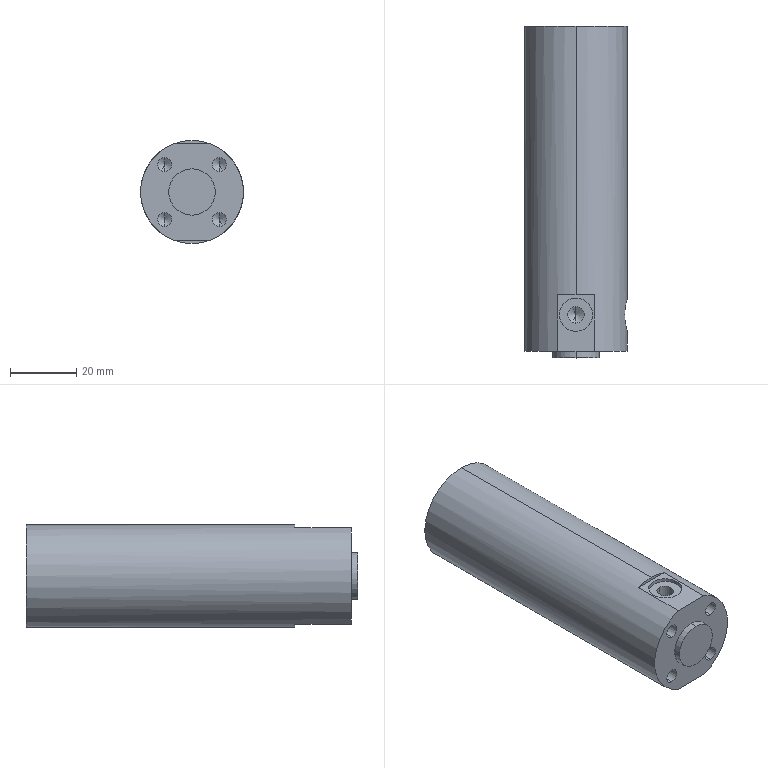Part | STEP file | 0229_Z_Cylinder_CG1BN25-50_1 | 1 solid | 54 faces | box 31 x 100 x 31 mm | volume 43980 mm3 | cylinder 28 | cone 14 | plane 12 | commonest cylinder face diameters 4.2 x8 10 x8 5 x4 6.8 x2 14 x2 25 x2